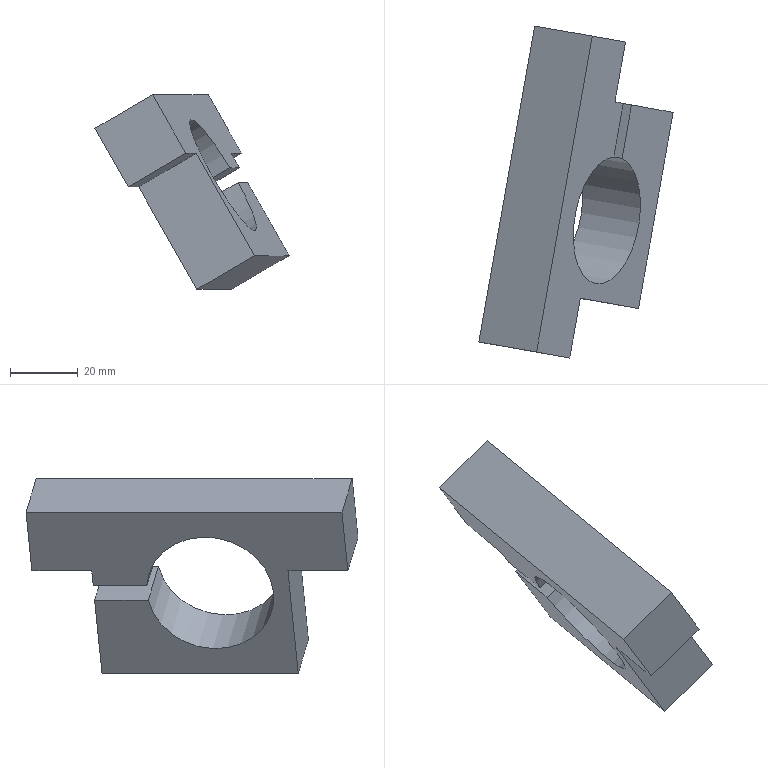Part | NX | features solid 2 | 1 solid | 14 faces | box 57.51 x 98.301 x 57.631 mm | volume 54898 mm3 | plane 13 | cylinder 1 | commonest cylinder face diameters 38.1 x1
STEP:
#1=CARTESIAN_POINT('',(-1020.919,60.813,-30.302));
#2=VERTEX_POINT('',#1);
#3=CARTESIAN_POINT('',(-1037.976,63.82,-40.302));
#4=VERTEX_POINT('',#3);
#5=CARTESIAN_POINT('',(-1037.976,63.82,-40.302));
#6=DIRECTION('',(-0.8529,0.1504,-0.5));
#7=VECTOR('',#6,1000.);
#8=LINE('',#5,#7);
#9=EDGE_CURVE('',#2,#4,#8,.T.);
#10=ORIENTED_EDGE('',*,*,#9,.F.);
#11=CARTESIAN_POINT('',(-1008.609,58.642,-51.953));
#12=VERTEX_POINT('',#11);
#13=CARTESIAN_POINT('',(-1030.767,62.549,-12.982));
#14=DIRECTION('',(0.4924,-0.08682,-0.866));
#15=VECTOR('',#14,1000.);
#16=LINE('',#13,#15);
#17=EDGE_CURVE('',#2,#12,#16,.T.);
#18=ORIENTED_EDGE('',*,*,#17,.T.);
#19=CARTESIAN_POINT('',(-1025.666,61.65,-61.953));
#20=VERTEX_POINT('',#19);
#21=CARTESIAN_POINT('',(-1025.666,61.65,-61.953));
#22=DIRECTION('',(0.8529,-0.1504,0.5));
#23=VECTOR('',#22,1000.);
#24=LINE('',#21,#23);
#25=EDGE_CURVE('',#20,#12,#24,.T.);
#26=ORIENTED_EDGE('',*,*,#25,.F.);
#27=CARTESIAN_POINT('',(-1047.824,65.557,-22.982));
#28=DIRECTION('',(0.4924,-0.08682,-0.866));
#29=VECTOR('',#28,1000.);
#30=LINE('',#27,#29);
#31=EDGE_CURVE('',#4,#20,#30,.T.);
#32=ORIENTED_EDGE('',*,*,#31,.F.);
#33=EDGE_LOOP('',(#10,#18,#26,#32));
#34=FACE_BOUND('',#33,.T.);
#35=CARTESIAN_POINT('',(-1047.824,65.557,-22.982));
#36=DIRECTION('',(-0.1736,-0.9848,0.));
#37=DIRECTION('',(-0.4924,0.08682,0.866));
#38=AXIS2_PLACEMENT_3D('',#35,#36,#37);
#39=PLANE('',#38);
#40=ADVANCED_FACE('',(#34),#39,.F.);
#41=ORIENTED_EDGE('',*,*,#25,.T.);
#42=CARTESIAN_POINT('',(-1018.854,0.5386,-51.953));
#43=VERTEX_POINT('',#42);
#44=CARTESIAN_POINT('',(-1009.39,54.211,-51.953));
#45=DIRECTION('',(-0.1736,-0.9848,0.));
#46=VECTOR('',#45,1000.);
#47=LINE('',#44,#46);
#48=EDGE_CURVE('',#12,#43,#47,.T.);
#49=ORIENTED_EDGE('',*,*,#48,.T.);
#50=CARTESIAN_POINT('',(-1035.911,3.546,-61.953));
#51=VERTEX_POINT('',#50);
#52=CARTESIAN_POINT('',(-1035.911,3.546,-61.953));
#53=DIRECTION('',(0.8529,-0.1504,0.5));
#54=VECTOR('',#53,1000.);
#55=LINE('',#52,#54);
#56=EDGE_CURVE('',#51,#43,#55,.T.);
#57=ORIENTED_EDGE('',*,*,#56,.F.);
#58=CARTESIAN_POINT('',(-1026.447,57.218,-61.953));
#59=DIRECTION('',(-0.1736,-0.9848,0.));
#60=VECTOR('',#59,1000.);
#61=LINE('',#58,#60);
#62=EDGE_CURVE('',#20,#51,#61,.T.);
#63=ORIENTED_EDGE('',*,*,#62,.F.);
#64=EDGE_LOOP('',(#41,#49,#57,#63));
#65=FACE_BOUND('',#64,.T.);
#66=CARTESIAN_POINT('',(-1026.447,57.218,-61.953));
#67=DIRECTION('',(-0.4924,0.08682,0.866));
#68=DIRECTION('',(0.1736,0.9848,0.));
#69=AXIS2_PLACEMENT_3D('',#66,#67,#68);
#70=PLANE('',#69);
#71=ADVANCED_FACE('',(#65),#70,.F.);
#72=CARTESIAN_POINT('',(-1025.843,61.681,-21.642));
#73=VERTEX_POINT('',#72);
#74=CARTESIAN_POINT('',(-1023.381,61.247,-25.972));
#75=VERTEX_POINT('',#74);
#76=CARTESIAN_POINT('',(-1030.767,62.549,-12.982));
#77=DIRECTION('',(0.4924,-0.08682,-0.866));
#78=VECTOR('',#77,1000.);
#79=LINE('',#76,#78);
#80=EDGE_CURVE('',#73,#75,#79,.T.);
#81=ORIENTED_EDGE('',*,*,#80,.T.);
#82=CARTESIAN_POINT('',(-1040.438,64.255,-35.972));
#83=VERTEX_POINT('',#82);
#84=CARTESIAN_POINT('',(-1040.438,64.255,-35.972));
#85=DIRECTION('',(-0.8529,0.1504,-0.5));
#86=VECTOR('',#85,1000.);
#87=LINE('',#84,#86);
#88=EDGE_CURVE('',#75,#83,#87,.T.);
#89=ORIENTED_EDGE('',*,*,#88,.T.);
#90=CARTESIAN_POINT('',(-1042.9,64.689,-31.642));
#91=VERTEX_POINT('',#90);
#92=CARTESIAN_POINT('',(-1047.824,65.557,-22.982));
#93=DIRECTION('',(0.4924,-0.08682,-0.866));
#94=VECTOR('',#93,1000.);
#95=LINE('',#92,#94);
#96=EDGE_CURVE('',#91,#83,#95,.T.);
#97=ORIENTED_EDGE('',*,*,#96,.F.);
#98=CARTESIAN_POINT('',(-1042.9,64.689,-31.642));
#99=DIRECTION('',(0.8529,-0.1504,0.5));
#100=VECTOR('',#99,1000.);
#101=LINE('',#98,#100);
#102=EDGE_CURVE('',#91,#73,#101,.T.);
#103=ORIENTED_EDGE('',*,*,#102,.T.);
#104=EDGE_LOOP('',(#81,#89,#97,#103));
#105=FACE_BOUND('',#104,.T.);
#106=CARTESIAN_POINT('',(-1047.824,65.557,-22.982));
#107=DIRECTION('',(-0.1736,-0.9848,0.));
#108=DIRECTION('',(-0.4924,0.08682,0.866));
#109=AXIS2_PLACEMENT_3D('',#106,#107,#108);
#110=PLANE('',#109);
#111=ADVANCED_FACE('',(#105),#110,.F.);
#112=CARTESIAN_POINT('',(-1053.145,6.585,-31.642));
#113=VERTEX_POINT('',#112);
#114=CARTESIAN_POINT('',(-1036.088,3.577,-21.642));
#115=VERTEX_POINT('',#114);
#116=CARTESIAN_POINT('',(-1053.145,6.585,-31.642));
#117=DIRECTION('',(0.8529,-0.1504,0.5));
#118=VECTOR('',#117,1000.);
#119=LINE('',#116,#118);
#120=EDGE_CURVE('',#113,#115,#119,.T.);
#121=ORIENTED_EDGE('',*,*,#120,.F.);
#122=CARTESIAN_POINT('',(-1058.069,7.453,-22.982));
#123=DIRECTION('',(0.4924,-0.08682,-0.866));
#124=VECTOR('',#123,1000.);
#125=LINE('',#122,#124);
#126=EDGE_CURVE('',#113,#51,#125,.T.);
#127=ORIENTED_EDGE('',*,*,#126,.T.);
#128=ORIENTED_EDGE('',*,*,#56,.T.);
#129=CARTESIAN_POINT('',(-1041.012,4.446,-12.982));
#130=DIRECTION('',(0.4924,-0.08682,-0.866));
#131=VECTOR('',#130,1000.);
#132=LINE('',#129,#131);
#133=EDGE_CURVE('',#115,#43,#132,.T.);
#134=ORIENTED_EDGE('',*,*,#133,.F.);
#135=EDGE_LOOP('',(#121,#127,#128,#134));
#136=FACE_BOUND('',#135,.T.);
#137=CARTESIAN_POINT('',(-1058.069,7.453,-22.982));
#138=DIRECTION('',(-0.1736,-0.9848,0.));
#139=DIRECTION('',(-0.4924,0.08682,0.866));
#140=AXIS2_PLACEMENT_3D('',#137,#138,#139);
#141=PLANE('',#140);
#142=ADVANCED_FACE('',(#136),#141,.T.);
#143=CARTESIAN_POINT('',(-1066.119,-9.405,-14.321));
#144=VERTEX_POINT('',#143);
#145=CARTESIAN_POINT('',(-1049.062,-12.413,-4.321));
#146=VERTEX_POINT('',#145);
#147=CARTESIAN_POINT('',(-1066.119,-9.405,-14.321));
#148=DIRECTION('',(-0.8529,0.1504,-0.5));
#149=VECTOR('',#148,1000.);
#150=LINE('',#147,#149);
#151=EDGE_CURVE('',#144,#146,#150,.F.);
#152=ORIENTED_EDGE('',*,*,#151,.T.);
#153=CARTESIAN_POINT('',(-1032.565,81.144,-4.321));
#154=VERTEX_POINT('',#153);
#155=CARTESIAN_POINT('',(-1036.472,58.986,-4.321));
#156=DIRECTION('',(-0.1736,-0.9848,0.));
#157=VECTOR('',#156,1000.);
#158=LINE('',#155,#157);
#159=EDGE_CURVE('',#154,#146,#158,.T.);
#160=ORIENTED_EDGE('',*,*,#159,.F.);
#161=CARTESIAN_POINT('',(-1049.622,84.152,-14.321));
#162=VERTEX_POINT('',#161);
#163=CARTESIAN_POINT('',(-1049.622,84.152,-14.321));
#164=DIRECTION('',(0.8529,-0.1504,0.5));
#165=VECTOR('',#164,1000.);
#166=LINE('',#163,#165);
#167=EDGE_CURVE('',#162,#154,#166,.T.);
#168=ORIENTED_EDGE('',*,*,#167,.F.);
#169=CARTESIAN_POINT('',(-1053.53,61.994,-14.321));
#170=DIRECTION('',(-0.1736,-0.9848,0.));
#171=VECTOR('',#170,1000.);
#172=LINE('',#169,#171);
#173=EDGE_CURVE('',#162,#144,#172,.T.);
#174=ORIENTED_EDGE('',*,*,#173,.T.);
#175=EDGE_LOOP('',(#152,#160,#168,#174));
#176=FACE_BOUND('',#175,.T.);
#177=CARTESIAN_POINT('',(-1053.53,61.994,-14.321));
#178=DIRECTION('',(-0.4924,0.08682,0.866));
#179=DIRECTION('',(0.1736,0.9848,0.));
#180=AXIS2_PLACEMENT_3D('',#177,#178,#179);
#181=PLANE('',#180);
#182=ADVANCED_FACE('',(#176),#181,.T.);
#183=CARTESIAN_POINT('',(-1043.236,48.385,-35.972));
#184=VERTEX_POINT('',#183);
#185=CARTESIAN_POINT('',(-1041.219,59.823,-35.972));
#186=DIRECTION('',(0.1736,0.9848,0.));
#187=VECTOR('',#186,1000.);
#188=LINE('',#185,#187);
#189=EDGE_CURVE('',#184,#83,#188,.T.);
#190=ORIENTED_EDGE('',*,*,#189,.F.);
#191=CARTESIAN_POINT('',(-1040.774,47.951,-40.302));
#192=VERTEX_POINT('',#191);
#193=CARTESIAN_POINT('',(-1045.285,29.569,-38.137));
#194=DIRECTION('',(0.8529,-0.1504,0.5));
#195=DIRECTION('',(-0.4924,0.08682,0.866));
#196=AXIS2_PLACEMENT_3D('',#193,#194,#195);
#197=CIRCLE('',#196,19.05);
#198=EDGE_CURVE('',#184,#192,#197,.T.);
#199=ORIENTED_EDGE('',*,*,#198,.T.);
#200=CARTESIAN_POINT('',(-1038.757,59.389,-40.302));
#201=DIRECTION('',(0.1736,0.9848,0.));
#202=VECTOR('',#201,1000.);
#203=LINE('',#200,#202);
#204=EDGE_CURVE('',#192,#4,#203,.T.);
#205=ORIENTED_EDGE('',*,*,#204,.T.);
#206=ORIENTED_EDGE('',*,*,#31,.T.);
#207=ORIENTED_EDGE('',*,*,#62,.T.);
#208=ORIENTED_EDGE('',*,*,#126,.F.);
#209=CARTESIAN_POINT('',(-1056.271,-11.141,-31.642));
#210=VERTEX_POINT('',#209);
#211=CARTESIAN_POINT('',(-1043.681,60.257,-31.642));
#212=DIRECTION('',(0.1736,0.9848,0.));
#213=VECTOR('',#212,1000.);
#214=LINE('',#211,#213);
#215=EDGE_CURVE('',#210,#113,#214,.T.);
#216=ORIENTED_EDGE('',*,*,#215,.F.);
#217=CARTESIAN_POINT('',(-1035.59,-14.788,-68.015));
#218=DIRECTION('',(-0.4924,0.08682,0.866));
#219=VECTOR('',#218,1000.);
#220=LINE('',#217,#219);
#221=EDGE_CURVE('',#144,#210,#220,.F.);
#222=ORIENTED_EDGE('',*,*,#221,.F.);
#223=ORIENTED_EDGE('',*,*,#173,.F.);
#224=CARTESIAN_POINT('',(-1039.774,82.415,-31.642));
#225=VERTEX_POINT('',#224);
#226=CARTESIAN_POINT('',(-1044.698,83.284,-22.982));
#227=DIRECTION('',(0.4924,-0.08682,-0.866));
#228=VECTOR('',#227,1000.);
#229=LINE('',#226,#228);
#230=EDGE_CURVE('',#162,#225,#229,.T.);
#231=ORIENTED_EDGE('',*,*,#230,.T.);
#232=CARTESIAN_POINT('',(-1043.681,60.257,-31.642));
#233=DIRECTION('',(0.1736,0.9848,0.));
#234=VECTOR('',#233,1000.);
#235=LINE('',#232,#234);
#236=EDGE_CURVE('',#91,#225,#235,.T.);
#237=ORIENTED_EDGE('',*,*,#236,.F.);
#238=ORIENTED_EDGE('',*,*,#96,.T.);
#239=EDGE_LOOP('',(#190,#199,#205,#206,#207,#208,#216,#222,#223,#231,#237,#238));
#240=FACE_BOUND('',#239,.T.);
#241=CARTESIAN_POINT('',(-1023.001,56.61,-68.015));
#242=DIRECTION('',(-0.8529,0.1504,-0.5));
#243=DIRECTION('',(-0.4924,0.08682,0.866));
#244=AXIS2_PLACEMENT_3D('',#241,#242,#243);
#245=PLANE('',#244);
#246=ADVANCED_FACE('',(#240),#245,.T.);
#247=CARTESIAN_POINT('',(-1023.717,44.943,-30.302));
#248=VERTEX_POINT('',#247);
#249=CARTESIAN_POINT('',(-1026.179,45.377,-25.972));
#250=VERTEX_POINT('',#249);
#251=CARTESIAN_POINT('',(-1028.227,26.562,-28.137));
#252=DIRECTION('',(-0.8529,0.1504,-0.5));
#253=DIRECTION('',(0.4924,-0.08682,-0.866));
#254=AXIS2_PLACEMENT_3D('',#251,#252,#253);
#255=CIRCLE('',#254,19.05);
#256=EDGE_CURVE('',#248,#250,#255,.T.);
#257=ORIENTED_EDGE('',*,*,#256,.T.);
#258=CARTESIAN_POINT('',(-1024.162,56.815,-25.972));
#259=DIRECTION('',(0.1736,0.9848,0.));
#260=VECTOR('',#259,1000.);
#261=LINE('',#258,#260);
#262=EDGE_CURVE('',#250,#75,#261,.T.);
#263=ORIENTED_EDGE('',*,*,#262,.T.);
#264=ORIENTED_EDGE('',*,*,#80,.F.);
#265=CARTESIAN_POINT('',(-1022.717,79.408,-21.642));
#266=VERTEX_POINT('',#265);
#267=CARTESIAN_POINT('',(-1026.624,57.249,-21.642));
#268=DIRECTION('',(0.1736,0.9848,0.));
#269=VECTOR('',#268,1000.);
#270=LINE('',#267,#269);
#271=EDGE_CURVE('',#73,#266,#270,.T.);
#272=ORIENTED_EDGE('',*,*,#271,.T.);
#273=CARTESIAN_POINT('',(-1027.641,80.276,-12.982));
#274=DIRECTION('',(0.4924,-0.08682,-0.866));
#275=VECTOR('',#274,1000.);
#276=LINE('',#273,#275);
#277=EDGE_CURVE('',#154,#266,#276,.T.);
#278=ORIENTED_EDGE('',*,*,#277,.F.);
#279=ORIENTED_EDGE('',*,*,#159,.T.);
#280=CARTESIAN_POINT('',(-1039.214,-14.149,-21.642));
#281=VERTEX_POINT('',#280);
#282=CARTESIAN_POINT('',(-1018.533,-17.796,-58.015));
#283=DIRECTION('',(-0.4924,0.08682,0.866));
#284=VECTOR('',#283,1000.);
#285=LINE('',#282,#284);
#286=EDGE_CURVE('',#146,#281,#285,.F.);
#287=ORIENTED_EDGE('',*,*,#286,.T.);
#288=CARTESIAN_POINT('',(-1026.624,57.249,-21.642));
#289=DIRECTION('',(0.1736,0.9848,0.));
#290=VECTOR('',#289,1000.);
#291=LINE('',#288,#290);
#292=EDGE_CURVE('',#281,#115,#291,.T.);
#293=ORIENTED_EDGE('',*,*,#292,.T.);
#294=ORIENTED_EDGE('',*,*,#133,.T.);
#295=ORIENTED_EDGE('',*,*,#48,.F.);
#296=ORIENTED_EDGE('',*,*,#17,.F.);
#297=CARTESIAN_POINT('',(-1021.7,56.381,-30.302));
#298=DIRECTION('',(0.1736,0.9848,0.));
#299=VECTOR('',#298,1000.);
#300=LINE('',#297,#299);
#301=EDGE_CURVE('',#248,#2,#300,.T.);
#302=ORIENTED_EDGE('',*,*,#301,.F.);
#303=EDGE_LOOP('',(#257,#263,#264,#272,#278,#279,#287,#293,#294,#295,#296,#302));
#304=FACE_BOUND('',#303,.T.);
#305=CARTESIAN_POINT('',(-1005.943,53.603,-58.015));
#306=DIRECTION('',(-0.8529,0.1504,-0.5));
#307=DIRECTION('',(-0.4924,0.08682,0.866));
#308=AXIS2_PLACEMENT_3D('',#305,#306,#307);
#309=PLANE('',#308);
#310=ADVANCED_FACE('',(#304),#309,.F.);
#311=ORIENTED_EDGE('',*,*,#277,.T.);
#312=CARTESIAN_POINT('',(-1039.774,82.415,-31.642));
#313=DIRECTION('',(0.8529,-0.1504,0.5));
#314=VECTOR('',#313,1000.);
#315=LINE('',#312,#314);
#316=EDGE_CURVE('',#225,#266,#315,.T.);
#317=ORIENTED_EDGE('',*,*,#316,.F.);
#318=ORIENTED_EDGE('',*,*,#230,.F.);
#319=ORIENTED_EDGE('',*,*,#167,.T.);
#320=EDGE_LOOP('',(#311,#317,#318,#319));
#321=FACE_BOUND('',#320,.T.);
#322=CARTESIAN_POINT('',(-1044.698,83.284,-22.982));
#323=DIRECTION('',(-0.1736,-0.9848,0.));
#324=DIRECTION('',(0.8529,-0.1504,0.5));
#325=AXIS2_PLACEMENT_3D('',#322,#323,#324);
#326=PLANE('',#325);
#327=ADVANCED_FACE('',(#321),#326,.F.);
#328=ORIENTED_EDGE('',*,*,#316,.T.);
#329=ORIENTED_EDGE('',*,*,#271,.F.);
#330=ORIENTED_EDGE('',*,*,#102,.F.);
#331=ORIENTED_EDGE('',*,*,#236,.T.);
#332=EDGE_LOOP('',(#328,#329,#330,#331));
#333=FACE_BOUND('',#332,.T.);
#334=CARTESIAN_POINT('',(-1043.681,60.257,-31.642));
#335=DIRECTION('',(-0.4924,0.08682,0.866));
#336=DIRECTION('',(-0.8529,0.1504,-0.5));
#337=AXIS2_PLACEMENT_3D('',#334,#335,#336);
#338=PLANE('',#337);
#339=ADVANCED_FACE('',(#333),#338,.F.);
#340=ORIENTED_EDGE('',*,*,#221,.T.);
#341=CARTESIAN_POINT('',(-1056.271,-11.141,-31.642));
#342=DIRECTION('',(-0.8529,0.1504,-0.5));
#343=VECTOR('',#342,1000.);
#344=LINE('',#341,#343);
#345=EDGE_CURVE('',#210,#281,#344,.F.);
#346=ORIENTED_EDGE('',*,*,#345,.T.);
#347=ORIENTED_EDGE('',*,*,#286,.F.);
#348=ORIENTED_EDGE('',*,*,#151,.F.);
#349=EDGE_LOOP('',(#340,#346,#347,#348));
#350=FACE_BOUND('',#349,.T.);
#351=CARTESIAN_POINT('',(-1061.195,-10.273,-22.982));
#352=DIRECTION('',(-0.1736,-0.9848,0.));
#353=DIRECTION('',(0.8529,-0.1504,0.5));
#354=AXIS2_PLACEMENT_3D('',#351,#352,#353);
#355=PLANE('',#354);
#356=ADVANCED_FACE('',(#350),#355,.T.);
#357=ORIENTED_EDGE('',*,*,#120,.T.);
#358=ORIENTED_EDGE('',*,*,#292,.F.);
#359=ORIENTED_EDGE('',*,*,#345,.F.);
#360=ORIENTED_EDGE('',*,*,#215,.T.);
#361=EDGE_LOOP('',(#357,#358,#359,#360));
#362=FACE_BOUND('',#361,.T.);
#363=CARTESIAN_POINT('',(-1055.49,-6.71,-31.642));
#364=DIRECTION('',(-0.4924,0.08682,0.866));
#365=DIRECTION('',(-0.8529,0.1504,-0.5));
#366=AXIS2_PLACEMENT_3D('',#363,#364,#365);
#367=PLANE('',#366);
#368=ADVANCED_FACE('',(#362),#367,.F.);
#369=ORIENTED_EDGE('',*,*,#198,.F.);
#370=CARTESIAN_POINT('',(-1043.236,48.385,-35.972));
#371=DIRECTION('',(0.8529,-0.1504,0.5));
#372=VECTOR('',#371,1000.);
#373=LINE('',#370,#372);
#374=EDGE_CURVE('',#184,#250,#373,.T.);
#375=ORIENTED_EDGE('',*,*,#374,.T.);
#376=ORIENTED_EDGE('',*,*,#256,.F.);
#377=CARTESIAN_POINT('',(-1040.774,47.951,-40.302));
#378=DIRECTION('',(0.8529,-0.1504,0.5));
#379=VECTOR('',#378,1000.);
#380=LINE('',#377,#379);
#381=EDGE_CURVE('',#192,#248,#380,.T.);
#382=ORIENTED_EDGE('',*,*,#381,.F.);
#383=EDGE_LOOP('',(#369,#375,#376,#382));
#384=FACE_BOUND('',#383,.T.);
#385=CARTESIAN_POINT('',(-1045.285,29.569,-38.137));
#386=DIRECTION('',(0.8529,-0.1504,0.5));
#387=DIRECTION('',(-0.4924,0.08682,0.866));
#388=AXIS2_PLACEMENT_3D('',#385,#386,#387);
#389=CYLINDRICAL_SURFACE('',#388,19.05);
#390=ADVANCED_FACE('',(#384),#389,.F.);
#391=ORIENTED_EDGE('',*,*,#9,.T.);
#392=ORIENTED_EDGE('',*,*,#204,.F.);
#393=ORIENTED_EDGE('',*,*,#381,.T.);
#394=ORIENTED_EDGE('',*,*,#301,.T.);
#395=EDGE_LOOP('',(#391,#392,#393,#394));
#396=FACE_BOUND('',#395,.T.);
#397=CARTESIAN_POINT('',(-958.767,14.314,9.698));
#398=DIRECTION('',(-0.4924,0.08682,0.866));
#399=DIRECTION('',(-0.8529,0.1504,-0.5));
#400=AXIS2_PLACEMENT_3D('',#397,#398,#399);
#401=PLANE('',#400);
#402=ADVANCED_FACE('',(#396),#401,.T.);
#403=ORIENTED_EDGE('',*,*,#262,.F.);
#404=ORIENTED_EDGE('',*,*,#374,.F.);
#405=ORIENTED_EDGE('',*,*,#189,.T.);
#406=ORIENTED_EDGE('',*,*,#88,.F.);
#407=EDGE_LOOP('',(#403,#404,#405,#406));
#408=FACE_BOUND('',#407,.T.);
#409=CARTESIAN_POINT('',(-961.229,14.748,14.028));
#410=DIRECTION('',(-0.4924,0.08682,0.866));
#411=DIRECTION('',(-0.8529,0.1504,-0.5));
#412=AXIS2_PLACEMENT_3D('',#409,#410,#411);
#413=PLANE('',#412);
#414=ADVANCED_FACE('',(#408),#413,.F.);
#415=CLOSED_SHELL('',(#40,#71,#111,#142,#182,#246,#310,#327,#339,#356,#368,#390,#402,#414));
#416=MANIFOLD_SOLID_BREP('',#415);
#417=(LENGTH_UNIT()NAMED_UNIT(*)SI_UNIT(.MILLI.,.METRE.));
#418=UNCERTAINTY_MEASURE_WITH_UNIT(LENGTH_MEASURE(0.00001),#417,'','');
#419=(NAMED_UNIT(*)PLANE_ANGLE_UNIT()SI_UNIT($,.RADIAN.));
#420=(NAMED_UNIT(*)SI_UNIT($,.STERADIAN.)SOLID_ANGLE_UNIT());
#421=(GEOMETRIC_REPRESENTATION_CONTEXT(3)GLOBAL_UNCERTAINTY_ASSIGNED_CONTEXT((#418))GLOBAL_UNIT_ASSIGNED_CONTEXT((#417,#419,#420))REPRESENTATION_CONTEXT('',''));
#422=ADVANCED_BREP_SHAPE_REPRESENTATION('',(#416),#421);